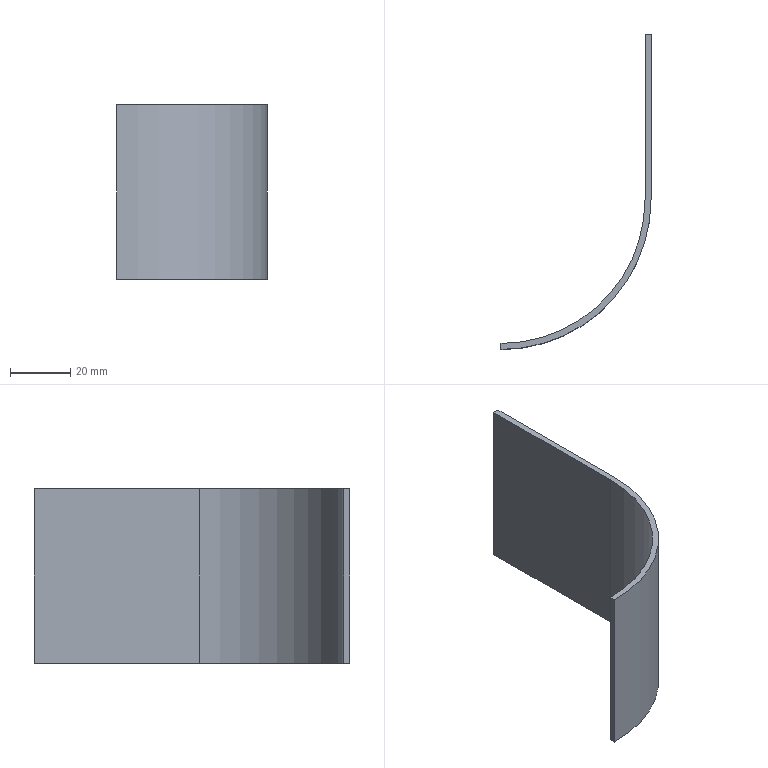Part | NX | features solid 2 | 1 solid | 8 faces | box 50 x 105 x 58 mm | volume 15308 mm3 | plane 6 | cylinder 2 | commonest cylinder face diameters 96 x1 100 x1
STEP:
#1=CARTESIAN_POINT('',(-402.,-1635.,965.));
#2=VERTEX_POINT('',#1);
#3=CARTESIAN_POINT('',(-450.,-1683.,965.));
#4=VERTEX_POINT('',#3);
#5=CARTESIAN_POINT('',(-450.,-1635.,965.));
#6=DIRECTION('',(0.,0.,-1.));
#7=DIRECTION('',(0.,-1.,0.));
#8=AXIS2_PLACEMENT_3D('',#5,#6,#7);
#9=CIRCLE('',#8,48.);
#10=EDGE_CURVE('',#2,#4,#9,.T.);
#11=ORIENTED_EDGE('',*,*,#10,.T.);
#12=CARTESIAN_POINT('',(-450.,-1683.,1023.));
#13=VERTEX_POINT('',#12);
#14=CARTESIAN_POINT('',(-450.,-1683.,1023.));
#15=DIRECTION('',(0.,0.,-1.));
#16=VECTOR('',#15,1000.);
#17=LINE('',#14,#16);
#18=EDGE_CURVE('',#13,#4,#17,.T.);
#19=ORIENTED_EDGE('',*,*,#18,.F.);
#20=CARTESIAN_POINT('',(-402.,-1635.,1023.));
#21=VERTEX_POINT('',#20);
#22=CARTESIAN_POINT('',(-450.,-1635.,1023.));
#23=DIRECTION('',(0.,0.,-1.));
#24=DIRECTION('',(0.,-1.,0.));
#25=AXIS2_PLACEMENT_3D('',#22,#23,#24);
#26=CIRCLE('',#25,48.);
#27=EDGE_CURVE('',#21,#13,#26,.T.);
#28=ORIENTED_EDGE('',*,*,#27,.F.);
#29=CARTESIAN_POINT('',(-402.,-1635.,1023.));
#30=DIRECTION('',(0.,0.,-1.));
#31=VECTOR('',#30,1000.);
#32=LINE('',#29,#31);
#33=EDGE_CURVE('',#21,#2,#32,.T.);
#34=ORIENTED_EDGE('',*,*,#33,.T.);
#35=EDGE_LOOP('',(#11,#19,#28,#34));
#36=FACE_BOUND('',#35,.T.);
#37=CARTESIAN_POINT('',(-450.,-1635.,1023.));
#38=DIRECTION('',(0.,0.,-1.));
#39=DIRECTION('',(0.,-1.,0.));
#40=AXIS2_PLACEMENT_3D('',#37,#38,#39);
#41=CYLINDRICAL_SURFACE('',#40,48.);
#42=ADVANCED_FACE('',(#36),#41,.F.);
#43=CARTESIAN_POINT('',(-402.,-1580.,965.));
#44=VERTEX_POINT('',#43);
#45=CARTESIAN_POINT('',(-402.,-1635.,965.));
#46=DIRECTION('',(0.,-1.,0.));
#47=VECTOR('',#46,1000.);
#48=LINE('',#45,#47);
#49=EDGE_CURVE('',#44,#2,#48,.T.);
#50=ORIENTED_EDGE('',*,*,#49,.T.);
#51=ORIENTED_EDGE('',*,*,#33,.F.);
#52=CARTESIAN_POINT('',(-402.,-1580.,1023.));
#53=VERTEX_POINT('',#52);
#54=CARTESIAN_POINT('',(-402.,-1635.,1023.));
#55=DIRECTION('',(0.,-1.,0.));
#56=VECTOR('',#55,1000.);
#57=LINE('',#54,#56);
#58=EDGE_CURVE('',#53,#21,#57,.T.);
#59=ORIENTED_EDGE('',*,*,#58,.F.);
#60=CARTESIAN_POINT('',(-402.,-1580.,1023.));
#61=DIRECTION('',(0.,0.,-1.));
#62=VECTOR('',#61,1000.);
#63=LINE('',#60,#62);
#64=EDGE_CURVE('',#53,#44,#63,.T.);
#65=ORIENTED_EDGE('',*,*,#64,.T.);
#66=EDGE_LOOP('',(#50,#51,#59,#65));
#67=FACE_BOUND('',#66,.T.);
#68=CARTESIAN_POINT('',(-402.,-1635.,1023.));
#69=DIRECTION('',(1.,0.,0.));
#70=DIRECTION('',(0.,0.,-1.));
#71=AXIS2_PLACEMENT_3D('',#68,#69,#70);
#72=PLANE('',#71);
#73=ADVANCED_FACE('',(#67),#72,.F.);
#74=ORIENTED_EDGE('',*,*,#64,.F.);
#75=CARTESIAN_POINT('',(-400.,-1580.,1023.));
#76=VERTEX_POINT('',#75);
#77=CARTESIAN_POINT('',(-400.,-1580.,1023.));
#78=DIRECTION('',(1.,0.,0.));
#79=VECTOR('',#78,1000.);
#80=LINE('',#77,#79);
#81=EDGE_CURVE('',#53,#76,#80,.T.);
#82=ORIENTED_EDGE('',*,*,#81,.T.);
#83=CARTESIAN_POINT('',(-400.,-1580.,965.));
#84=VERTEX_POINT('',#83);
#85=CARTESIAN_POINT('',(-400.,-1580.,1023.));
#86=DIRECTION('',(0.,0.,-1.));
#87=VECTOR('',#86,1000.);
#88=LINE('',#85,#87);
#89=EDGE_CURVE('',#76,#84,#88,.T.);
#90=ORIENTED_EDGE('',*,*,#89,.T.);
#91=CARTESIAN_POINT('',(-400.,-1580.,965.));
#92=DIRECTION('',(1.,0.,0.));
#93=VECTOR('',#92,1000.);
#94=LINE('',#91,#93);
#95=EDGE_CURVE('',#44,#84,#94,.T.);
#96=ORIENTED_EDGE('',*,*,#95,.F.);
#97=EDGE_LOOP('',(#74,#82,#90,#96));
#98=FACE_BOUND('',#97,.T.);
#99=CARTESIAN_POINT('',(-400.,-1580.,1023.));
#100=DIRECTION('',(0.,-1.,0.));
#101=DIRECTION('',(-1.,0.,0.));
#102=AXIS2_PLACEMENT_3D('',#99,#100,#101);
#103=PLANE('',#102);
#104=ADVANCED_FACE('',(#98),#103,.F.);
#105=CARTESIAN_POINT('',(-400.,-1635.,965.));
#106=VERTEX_POINT('',#105);
#107=CARTESIAN_POINT('',(-450.,-1685.,965.));
#108=VERTEX_POINT('',#107);
#109=CARTESIAN_POINT('',(-450.,-1635.,965.));
#110=DIRECTION('',(0.,0.,-1.));
#111=DIRECTION('',(0.,1.,0.));
#112=AXIS2_PLACEMENT_3D('',#109,#110,#111);
#113=CIRCLE('',#112,50.);
#114=EDGE_CURVE('',#106,#108,#113,.T.);
#115=ORIENTED_EDGE('',*,*,#114,.F.);
#116=CARTESIAN_POINT('',(-400.,-1635.,1023.));
#117=VERTEX_POINT('',#116);
#118=CARTESIAN_POINT('',(-400.,-1635.,1023.));
#119=DIRECTION('',(0.,0.,-1.));
#120=VECTOR('',#119,1000.);
#121=LINE('',#118,#120);
#122=EDGE_CURVE('',#117,#106,#121,.T.);
#123=ORIENTED_EDGE('',*,*,#122,.F.);
#124=CARTESIAN_POINT('',(-450.,-1685.,1023.));
#125=VERTEX_POINT('',#124);
#126=CARTESIAN_POINT('',(-450.,-1635.,1023.));
#127=DIRECTION('',(0.,0.,-1.));
#128=DIRECTION('',(0.,1.,0.));
#129=AXIS2_PLACEMENT_3D('',#126,#127,#128);
#130=CIRCLE('',#129,50.);
#131=EDGE_CURVE('',#117,#125,#130,.T.);
#132=ORIENTED_EDGE('',*,*,#131,.T.);
#133=CARTESIAN_POINT('',(-450.,-1685.,1023.));
#134=DIRECTION('',(0.,0.,-1.));
#135=VECTOR('',#134,1000.);
#136=LINE('',#133,#135);
#137=EDGE_CURVE('',#125,#108,#136,.T.);
#138=ORIENTED_EDGE('',*,*,#137,.T.);
#139=EDGE_LOOP('',(#115,#123,#132,#138));
#140=FACE_BOUND('',#139,.T.);
#141=CARTESIAN_POINT('',(-450.,-1635.,1023.));
#142=DIRECTION('',(0.,0.,-1.));
#143=DIRECTION('',(0.,-1.,0.));
#144=AXIS2_PLACEMENT_3D('',#141,#142,#143);
#145=CYLINDRICAL_SURFACE('',#144,50.);
#146=ADVANCED_FACE('',(#140),#145,.T.);
#147=CARTESIAN_POINT('',(-400.,-1635.,965.));
#148=DIRECTION('',(0.,-1.,0.));
#149=VECTOR('',#148,1000.);
#150=LINE('',#147,#149);
#151=EDGE_CURVE('',#84,#106,#150,.T.);
#152=ORIENTED_EDGE('',*,*,#151,.F.);
#153=ORIENTED_EDGE('',*,*,#89,.F.);
#154=CARTESIAN_POINT('',(-400.,-1635.,1023.));
#155=DIRECTION('',(0.,-1.,0.));
#156=VECTOR('',#155,1000.);
#157=LINE('',#154,#156);
#158=EDGE_CURVE('',#76,#117,#157,.T.);
#159=ORIENTED_EDGE('',*,*,#158,.T.);
#160=ORIENTED_EDGE('',*,*,#122,.T.);
#161=EDGE_LOOP('',(#152,#153,#159,#160));
#162=FACE_BOUND('',#161,.T.);
#163=CARTESIAN_POINT('',(-400.,-1635.,1023.));
#164=DIRECTION('',(1.,0.,0.));
#165=DIRECTION('',(0.,0.,-1.));
#166=AXIS2_PLACEMENT_3D('',#163,#164,#165);
#167=PLANE('',#166);
#168=ADVANCED_FACE('',(#162),#167,.T.);
#169=ORIENTED_EDGE('',*,*,#151,.T.);
#170=ORIENTED_EDGE('',*,*,#114,.T.);
#171=CARTESIAN_POINT('',(-450.,-1685.,965.));
#172=DIRECTION('',(0.,-1.,0.));
#173=VECTOR('',#172,1000.);
#174=LINE('',#171,#173);
#175=EDGE_CURVE('',#4,#108,#174,.T.);
#176=ORIENTED_EDGE('',*,*,#175,.F.);
#177=ORIENTED_EDGE('',*,*,#10,.F.);
#178=ORIENTED_EDGE('',*,*,#49,.F.);
#179=ORIENTED_EDGE('',*,*,#95,.T.);
#180=EDGE_LOOP('',(#169,#170,#176,#177,#178,#179));
#181=FACE_BOUND('',#180,.T.);
#182=CARTESIAN_POINT('',(-400.,-1635.,965.));
#183=DIRECTION('',(0.,0.,1.));
#184=DIRECTION('',(0.,-1.,0.));
#185=AXIS2_PLACEMENT_3D('',#182,#183,#184);
#186=PLANE('',#185);
#187=ADVANCED_FACE('',(#181),#186,.F.);
#188=CARTESIAN_POINT('',(-450.,-1685.,1023.));
#189=DIRECTION('',(0.,-1.,0.));
#190=VECTOR('',#189,1000.);
#191=LINE('',#188,#190);
#192=EDGE_CURVE('',#13,#125,#191,.T.);
#193=ORIENTED_EDGE('',*,*,#192,.F.);
#194=ORIENTED_EDGE('',*,*,#18,.T.);
#195=ORIENTED_EDGE('',*,*,#175,.T.);
#196=ORIENTED_EDGE('',*,*,#137,.F.);
#197=EDGE_LOOP('',(#193,#194,#195,#196));
#198=FACE_BOUND('',#197,.T.);
#199=CARTESIAN_POINT('',(-450.,-1685.,994.));
#200=DIRECTION('',(-1.,0.,0.));
#201=DIRECTION('',(0.,1.,0.));
#202=AXIS2_PLACEMENT_3D('',#199,#200,#201);
#203=PLANE('',#202);
#204=ADVANCED_FACE('',(#198),#203,.T.);
#205=ORIENTED_EDGE('',*,*,#131,.F.);
#206=ORIENTED_EDGE('',*,*,#158,.F.);
#207=ORIENTED_EDGE('',*,*,#81,.F.);
#208=ORIENTED_EDGE('',*,*,#58,.T.);
#209=ORIENTED_EDGE('',*,*,#27,.T.);
#210=ORIENTED_EDGE('',*,*,#192,.T.);
#211=EDGE_LOOP('',(#205,#206,#207,#208,#209,#210));
#212=FACE_BOUND('',#211,.T.);
#213=CARTESIAN_POINT('',(-450.,-1635.,1023.));
#214=DIRECTION('',(0.,0.,1.));
#215=DIRECTION('',(0.,-1.,0.));
#216=AXIS2_PLACEMENT_3D('',#213,#214,#215);
#217=PLANE('',#216);
#218=ADVANCED_FACE('',(#212),#217,.T.);
#219=CLOSED_SHELL('',(#42,#73,#104,#146,#168,#187,#204,#218));
#220=MANIFOLD_SOLID_BREP('',#219);
#221=(LENGTH_UNIT()NAMED_UNIT(*)SI_UNIT(.MILLI.,.METRE.));
#222=UNCERTAINTY_MEASURE_WITH_UNIT(LENGTH_MEASURE(0.00001),#221,'','');
#223=(NAMED_UNIT(*)PLANE_ANGLE_UNIT()SI_UNIT($,.RADIAN.));
#224=(NAMED_UNIT(*)SI_UNIT($,.STERADIAN.)SOLID_ANGLE_UNIT());
#225=(GEOMETRIC_REPRESENTATION_CONTEXT(3)GLOBAL_UNCERTAINTY_ASSIGNED_CONTEXT((#222))GLOBAL_UNIT_ASSIGNED_CONTEXT((#221,#223,#224))REPRESENTATION_CONTEXT('',''));
#226=ADVANCED_BREP_SHAPE_REPRESENTATION('',(#220),#225);